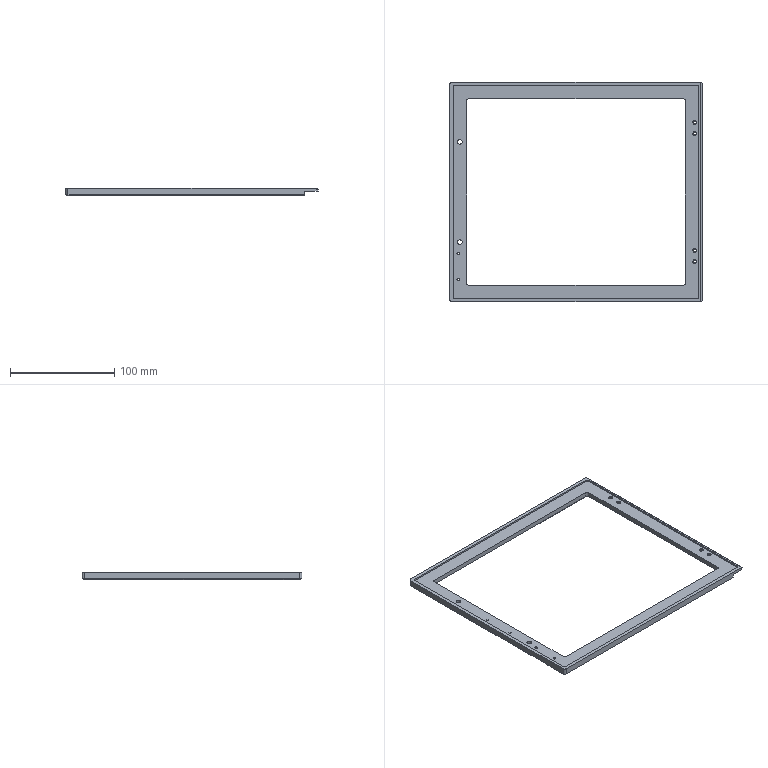Part | 1 solid | 107 faces | box 241.5 x 210.5 x 7 mm | volume 62907 mm3 | cylinder 45 | plane 40 | cone 22 | commonest cylinder face diameters 2 x10 2.5 x8 3.8 x8 4 x8 4.4 x4 4.5 x4